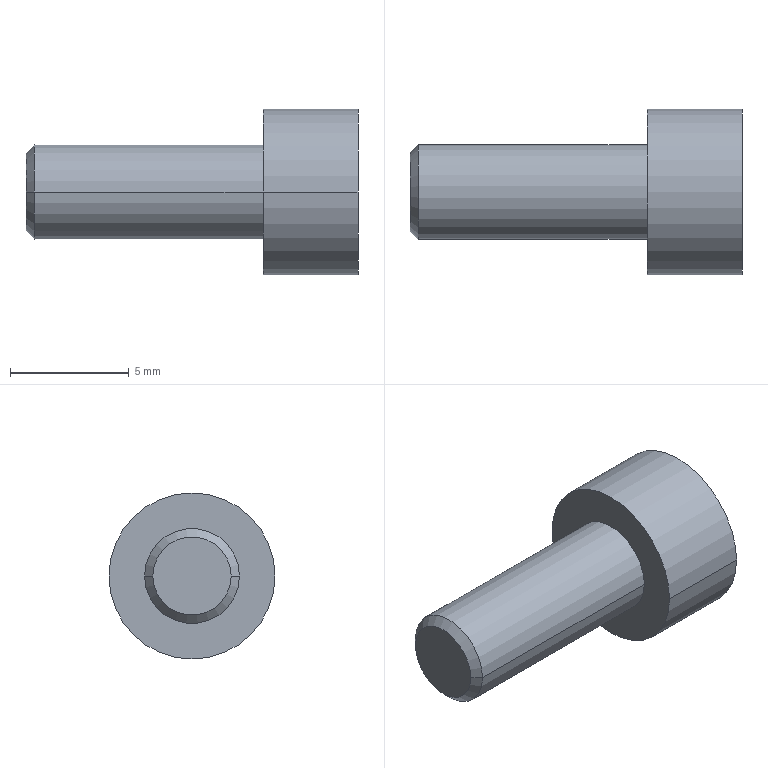Part | STEP file | 4-20.sldasm-Part-224 | 1 solid | 16 faces | box 14 x 7 x 7 mm | volume 258.3 mm3 | plane 10 | cylinder 4 | cone 2 | commonest cylinder face diameters 4 x2 7 x2
STEP:
#1=CARTESIAN_POINT('',(126.065,599.075,-92.493));
#2=VERTEX_POINT('',#1);
#3=CARTESIAN_POINT('',(126.065,595.775,-92.493));
#4=VERTEX_POINT('',#3);
#5=CARTESIAN_POINT('',(126.065,597.425,-92.493));
#6=DIRECTION('',(-1.,0.,0.));
#7=DIRECTION('',(0.,-1.,0.));
#8=AXIS2_PLACEMENT_3D('',#5,#6,#7);
#9=CIRCLE('',#8,1.65);
#10=EDGE_CURVE('',#2,#4,#9,.T.);
#11=ORIENTED_EDGE('',*,*,#10,.F.);
#12=CARTESIAN_POINT('',(126.415,599.425,-92.493));
#13=VERTEX_POINT('',#12);
#14=CARTESIAN_POINT('',(126.415,599.425,-92.493));
#15=DIRECTION('',(0.7071,0.7071,0.));
#16=VECTOR('',#15,1000.);
#17=LINE('',#14,#16);
#18=EDGE_CURVE('',#2,#13,#17,.T.);
#19=ORIENTED_EDGE('',*,*,#18,.T.);
#20=CARTESIAN_POINT('',(126.415,595.425,-92.493));
#21=VERTEX_POINT('',#20);
#22=CARTESIAN_POINT('',(126.415,597.425,-92.493));
#23=DIRECTION('',(1.,0.,0.));
#24=DIRECTION('',(0.,-1.,0.));
#25=AXIS2_PLACEMENT_3D('',#22,#23,#24);
#26=CIRCLE('',#25,2.);
#27=EDGE_CURVE('',#21,#13,#26,.T.);
#28=ORIENTED_EDGE('',*,*,#27,.F.);
#29=CARTESIAN_POINT('',(126.415,595.425,-92.493));
#30=DIRECTION('',(0.7071,-0.7071,0.));
#31=VECTOR('',#30,1000.);
#32=LINE('',#29,#31);
#33=EDGE_CURVE('',#4,#21,#32,.T.);
#34=ORIENTED_EDGE('',*,*,#33,.F.);
#35=EDGE_LOOP('',(#11,#19,#28,#34));
#36=FACE_OUTER_BOUND('',#35,.T.);
#37=CARTESIAN_POINT('',(126.415,597.425,-92.493));
#38=DIRECTION('',(1.,0.,0.));
#39=DIRECTION('',(0.,-1.,0.));
#40=AXIS2_PLACEMENT_3D('',#37,#38,#39);
#41=CONICAL_SURFACE('',#40,2.,0.7854);
#42=ADVANCED_FACE('',(#36),#41,.T.);
#43=CARTESIAN_POINT('',(136.065,593.925,-92.493));
#44=VERTEX_POINT('',#43);
#45=CARTESIAN_POINT('',(136.065,600.925,-92.493));
#46=VERTEX_POINT('',#45);
#47=CARTESIAN_POINT('',(136.065,597.425,-92.493));
#48=DIRECTION('',(1.,0.,0.));
#49=DIRECTION('',(0.,-1.,0.));
#50=AXIS2_PLACEMENT_3D('',#47,#48,#49);
#51=CIRCLE('',#50,3.5);
#52=EDGE_CURVE('',#44,#46,#51,.T.);
#53=ORIENTED_EDGE('',*,*,#52,.T.);
#54=CARTESIAN_POINT('',(140.065,600.925,-92.493));
#55=VERTEX_POINT('',#54);
#56=CARTESIAN_POINT('',(136.065,600.925,-92.493));
#57=DIRECTION('',(1.,0.,0.));
#58=VECTOR('',#57,1000.);
#59=LINE('',#56,#58);
#60=EDGE_CURVE('',#46,#55,#59,.T.);
#61=ORIENTED_EDGE('',*,*,#60,.T.);
#62=CARTESIAN_POINT('',(140.065,593.925,-92.493));
#63=VERTEX_POINT('',#62);
#64=CARTESIAN_POINT('',(140.065,597.425,-92.493));
#65=DIRECTION('',(1.,0.,0.));
#66=DIRECTION('',(0.,-1.,0.));
#67=AXIS2_PLACEMENT_3D('',#64,#65,#66);
#68=CIRCLE('',#67,3.5);
#69=EDGE_CURVE('',#63,#55,#68,.T.);
#70=ORIENTED_EDGE('',*,*,#69,.F.);
#71=CARTESIAN_POINT('',(136.065,593.925,-92.493));
#72=DIRECTION('',(1.,0.,0.));
#73=VECTOR('',#72,1000.);
#74=LINE('',#71,#73);
#75=EDGE_CURVE('',#44,#63,#74,.T.);
#76=ORIENTED_EDGE('',*,*,#75,.F.);
#77=EDGE_LOOP('',(#53,#61,#70,#76));
#78=FACE_OUTER_BOUND('',#77,.T.);
#79=CARTESIAN_POINT('',(136.065,597.425,-92.493));
#80=DIRECTION('',(1.,0.,0.));
#81=DIRECTION('',(0.,-1.,0.));
#82=AXIS2_PLACEMENT_3D('',#79,#80,#81);
#83=CYLINDRICAL_SURFACE('',#82,3.5);
#84=ADVANCED_FACE('',(#78),#83,.T.);
#85=CARTESIAN_POINT('',(136.065,595.425,-92.493));
#86=VERTEX_POINT('',#85);
#87=CARTESIAN_POINT('',(136.065,599.425,-92.493));
#88=VERTEX_POINT('',#87);
#89=CARTESIAN_POINT('',(136.065,597.425,-92.493));
#90=DIRECTION('',(1.,0.,0.));
#91=DIRECTION('',(0.,-1.,0.));
#92=AXIS2_PLACEMENT_3D('',#89,#90,#91);
#93=CIRCLE('',#92,2.);
#94=EDGE_CURVE('',#86,#88,#93,.T.);
#95=ORIENTED_EDGE('',*,*,#94,.F.);
#96=CARTESIAN_POINT('',(136.065,595.425,-92.493));
#97=DIRECTION('',(-1.,0.,0.));
#98=VECTOR('',#97,1000.);
#99=LINE('',#96,#98);
#100=EDGE_CURVE('',#86,#21,#99,.T.);
#101=ORIENTED_EDGE('',*,*,#100,.T.);
#102=ORIENTED_EDGE('',*,*,#27,.T.);
#103=CARTESIAN_POINT('',(136.065,599.425,-92.493));
#104=DIRECTION('',(-1.,0.,0.));
#105=VECTOR('',#104,1000.);
#106=LINE('',#103,#105);
#107=EDGE_CURVE('',#88,#13,#106,.T.);
#108=ORIENTED_EDGE('',*,*,#107,.F.);
#109=EDGE_LOOP('',(#95,#101,#102,#108));
#110=FACE_OUTER_BOUND('',#109,.T.);
#111=CARTESIAN_POINT('',(136.065,597.425,-92.493));
#112=DIRECTION('',(-1.,0.,0.));
#113=DIRECTION('',(0.,1.,0.));
#114=AXIS2_PLACEMENT_3D('',#111,#112,#113);
#115=CYLINDRICAL_SURFACE('',#114,2.);
#116=ADVANCED_FACE('',(#110),#115,.T.);
#117=ORIENTED_EDGE('',*,*,#100,.F.);
#118=CARTESIAN_POINT('',(136.065,597.425,-92.493));
#119=DIRECTION('',(1.,0.,0.));
#120=DIRECTION('',(0.,-1.,0.));
#121=AXIS2_PLACEMENT_3D('',#118,#119,#120);
#122=CIRCLE('',#121,2.);
#123=EDGE_CURVE('',#88,#86,#122,.T.);
#124=ORIENTED_EDGE('',*,*,#123,.F.);
#125=ORIENTED_EDGE('',*,*,#107,.T.);
#126=CARTESIAN_POINT('',(126.415,597.425,-92.493));
#127=DIRECTION('',(1.,0.,0.));
#128=DIRECTION('',(0.,-1.,0.));
#129=AXIS2_PLACEMENT_3D('',#126,#127,#128);
#130=CIRCLE('',#129,2.);
#131=EDGE_CURVE('',#13,#21,#130,.T.);
#132=ORIENTED_EDGE('',*,*,#131,.T.);
#133=EDGE_LOOP('',(#117,#124,#125,#132));
#134=FACE_OUTER_BOUND('',#133,.T.);
#135=CARTESIAN_POINT('',(136.065,597.425,-92.493));
#136=DIRECTION('',(-1.,0.,0.));
#137=DIRECTION('',(0.,1.,0.));
#138=AXIS2_PLACEMENT_3D('',#135,#136,#137);
#139=CYLINDRICAL_SURFACE('',#138,2.);
#140=ADVANCED_FACE('',(#134),#139,.T.);
#141=CARTESIAN_POINT('',(126.065,597.425,-92.493));
#142=DIRECTION('',(-1.,0.,0.));
#143=DIRECTION('',(0.,-1.,0.));
#144=AXIS2_PLACEMENT_3D('',#141,#142,#143);
#145=CIRCLE('',#144,1.65);
#146=EDGE_CURVE('',#4,#2,#145,.T.);
#147=ORIENTED_EDGE('',*,*,#146,.T.);
#148=ORIENTED_EDGE('',*,*,#10,.T.);
#149=EDGE_LOOP('',(#147,#148));
#150=FACE_OUTER_BOUND('',#149,.T.);
#151=CARTESIAN_POINT('',(126.065,597.425,-92.493));
#152=DIRECTION('',(1.,0.,0.));
#153=DIRECTION('',(0.,-1.,0.));
#154=AXIS2_PLACEMENT_3D('',#151,#152,#153);
#155=PLANE('',#154);
#156=ADVANCED_FACE('',(#150),#155,.F.);
#157=ORIENTED_EDGE('',*,*,#52,.F.);
#158=CARTESIAN_POINT('',(136.065,597.425,-92.493));
#159=DIRECTION('',(1.,0.,0.));
#160=DIRECTION('',(0.,-1.,0.));
#161=AXIS2_PLACEMENT_3D('',#158,#159,#160);
#162=CIRCLE('',#161,3.5);
#163=EDGE_CURVE('',#46,#44,#162,.T.);
#164=ORIENTED_EDGE('',*,*,#163,.F.);
#165=EDGE_LOOP('',(#157,#164));
#166=FACE_OUTER_BOUND('',#165,.T.);
#167=ORIENTED_EDGE('',*,*,#123,.T.);
#168=ORIENTED_EDGE('',*,*,#94,.T.);
#169=EDGE_LOOP('',(#167,#168));
#170=FACE_BOUND('',#169,.T.);
#171=CARTESIAN_POINT('',(136.065,597.425,-92.493));
#172=DIRECTION('',(-1.,0.,0.));
#173=DIRECTION('',(0.,1.,0.));
#174=AXIS2_PLACEMENT_3D('',#171,#172,#173);
#175=PLANE('',#174);
#176=ADVANCED_FACE('',(#166,#170),#175,.T.);
#177=CARTESIAN_POINT('',(140.065,598.291,-90.993));
#178=VERTEX_POINT('',#177);
#179=CARTESIAN_POINT('',(140.065,596.559,-90.993));
#180=VERTEX_POINT('',#179);
#181=CARTESIAN_POINT('',(140.065,598.291,-90.993));
#182=DIRECTION('',(0.,-1.,0.));
#183=VECTOR('',#182,1000.);
#184=LINE('',#181,#183);
#185=EDGE_CURVE('',#178,#180,#184,.T.);
#186=ORIENTED_EDGE('',*,*,#185,.F.);
#187=CARTESIAN_POINT('',(140.065,599.157,-92.493));
#188=VERTEX_POINT('',#187);
#189=CARTESIAN_POINT('',(140.065,599.157,-92.493));
#190=DIRECTION('',(0.,-0.5,0.866));
#191=VECTOR('',#190,1000.);
#192=LINE('',#189,#191);
#193=EDGE_CURVE('',#188,#178,#192,.T.);
#194=ORIENTED_EDGE('',*,*,#193,.F.);
#195=CARTESIAN_POINT('',(140.065,598.291,-93.993));
#196=VERTEX_POINT('',#195);
#197=CARTESIAN_POINT('',(140.065,598.291,-93.993));
#198=DIRECTION('',(0.,0.5,0.866));
#199=VECTOR('',#198,1000.);
#200=LINE('',#197,#199);
#201=EDGE_CURVE('',#196,#188,#200,.T.);
#202=ORIENTED_EDGE('',*,*,#201,.F.);
#203=CARTESIAN_POINT('',(140.065,596.559,-93.993));
#204=VERTEX_POINT('',#203);
#205=CARTESIAN_POINT('',(140.065,596.559,-93.993));
#206=DIRECTION('',(0.,1.,0.));
#207=VECTOR('',#206,1000.);
#208=LINE('',#205,#207);
#209=EDGE_CURVE('',#204,#196,#208,.T.);
#210=ORIENTED_EDGE('',*,*,#209,.F.);
#211=CARTESIAN_POINT('',(140.065,595.693,-92.493));
#212=VERTEX_POINT('',#211);
#213=CARTESIAN_POINT('',(140.065,595.693,-92.493));
#214=DIRECTION('',(0.,0.5,-0.866));
#215=VECTOR('',#214,1000.);
#216=LINE('',#213,#215);
#217=EDGE_CURVE('',#212,#204,#216,.T.);
#218=ORIENTED_EDGE('',*,*,#217,.F.);
#219=CARTESIAN_POINT('',(140.065,596.559,-90.993));
#220=DIRECTION('',(0.,-0.5,-0.866));
#221=VECTOR('',#220,1000.);
#222=LINE('',#219,#221);
#223=EDGE_CURVE('',#180,#212,#222,.T.);
#224=ORIENTED_EDGE('',*,*,#223,.F.);
#225=EDGE_LOOP('',(#186,#194,#202,#210,#218,#224));
#226=FACE_BOUND('',#225,.T.);
#227=ORIENTED_EDGE('',*,*,#69,.T.);
#228=CARTESIAN_POINT('',(140.065,597.425,-92.493));
#229=DIRECTION('',(1.,0.,0.));
#230=DIRECTION('',(0.,-1.,0.));
#231=AXIS2_PLACEMENT_3D('',#228,#229,#230);
#232=CIRCLE('',#231,3.5);
#233=EDGE_CURVE('',#55,#63,#232,.T.);
#234=ORIENTED_EDGE('',*,*,#233,.T.);
#235=EDGE_LOOP('',(#227,#234));
#236=FACE_OUTER_BOUND('',#235,.T.);
#237=CARTESIAN_POINT('',(140.065,597.425,-92.493));
#238=DIRECTION('',(1.,0.,0.));
#239=DIRECTION('',(0.,-1.,0.));
#240=AXIS2_PLACEMENT_3D('',#237,#238,#239);
#241=PLANE('',#240);
#242=ADVANCED_FACE('',(#226,#236),#241,.T.);
#243=ORIENTED_EDGE('',*,*,#60,.F.);
#244=ORIENTED_EDGE('',*,*,#163,.T.);
#245=ORIENTED_EDGE('',*,*,#75,.T.);
#246=ORIENTED_EDGE('',*,*,#233,.F.);
#247=EDGE_LOOP('',(#243,#244,#245,#246));
#248=FACE_OUTER_BOUND('',#247,.T.);
#249=CARTESIAN_POINT('',(136.065,597.425,-92.493));
#250=DIRECTION('',(1.,0.,0.));
#251=DIRECTION('',(0.,-1.,0.));
#252=AXIS2_PLACEMENT_3D('',#249,#250,#251);
#253=CYLINDRICAL_SURFACE('',#252,3.5);
#254=ADVANCED_FACE('',(#248),#253,.T.);
#255=ORIENTED_EDGE('',*,*,#18,.F.);
#256=ORIENTED_EDGE('',*,*,#146,.F.);
#257=ORIENTED_EDGE('',*,*,#33,.T.);
#258=ORIENTED_EDGE('',*,*,#131,.F.);
#259=EDGE_LOOP('',(#255,#256,#257,#258));
#260=FACE_OUTER_BOUND('',#259,.T.);
#261=CARTESIAN_POINT('',(126.415,597.425,-92.493));
#262=DIRECTION('',(1.,0.,0.));
#263=DIRECTION('',(0.,-1.,0.));
#264=AXIS2_PLACEMENT_3D('',#261,#262,#263);
#265=CONICAL_SURFACE('',#264,2.,0.7854);
#266=ADVANCED_FACE('',(#260),#265,.T.);
#267=ORIENTED_EDGE('',*,*,#185,.T.);
#268=CARTESIAN_POINT('',(137.425,596.559,-90.993));
#269=VERTEX_POINT('',#268);
#270=CARTESIAN_POINT('',(137.425,596.559,-90.993));
#271=DIRECTION('',(1.,0.,0.));
#272=VECTOR('',#271,1000.);
#273=LINE('',#270,#272);
#274=EDGE_CURVE('',#269,#180,#273,.T.);
#275=ORIENTED_EDGE('',*,*,#274,.F.);
#276=CARTESIAN_POINT('',(137.425,598.291,-90.993));
#277=VERTEX_POINT('',#276);
#278=CARTESIAN_POINT('',(137.425,598.291,-90.993));
#279=DIRECTION('',(0.,-1.,0.));
#280=VECTOR('',#279,1000.);
#281=LINE('',#278,#280);
#282=EDGE_CURVE('',#277,#269,#281,.T.);
#283=ORIENTED_EDGE('',*,*,#282,.F.);
#284=CARTESIAN_POINT('',(137.425,598.291,-90.993));
#285=DIRECTION('',(1.,0.,0.));
#286=VECTOR('',#285,1000.);
#287=LINE('',#284,#286);
#288=EDGE_CURVE('',#277,#178,#287,.T.);
#289=ORIENTED_EDGE('',*,*,#288,.T.);
#290=EDGE_LOOP('',(#267,#275,#283,#289));
#291=FACE_OUTER_BOUND('',#290,.T.);
#292=CARTESIAN_POINT('',(137.425,598.291,-90.993));
#293=DIRECTION('',(0.,0.,1.));
#294=DIRECTION('',(-1.,0.,0.));
#295=AXIS2_PLACEMENT_3D('',#292,#293,#294);
#296=PLANE('',#295);
#297=ADVANCED_FACE('',(#291),#296,.F.);
#298=ORIENTED_EDGE('',*,*,#223,.T.);
#299=CARTESIAN_POINT('',(137.425,595.693,-92.493));
#300=VERTEX_POINT('',#299);
#301=CARTESIAN_POINT('',(137.425,595.693,-92.493));
#302=DIRECTION('',(1.,0.,0.));
#303=VECTOR('',#302,1000.);
#304=LINE('',#301,#303);
#305=EDGE_CURVE('',#300,#212,#304,.T.);
#306=ORIENTED_EDGE('',*,*,#305,.F.);
#307=CARTESIAN_POINT('',(137.425,596.559,-90.993));
#308=DIRECTION('',(0.,-0.5,-0.866));
#309=VECTOR('',#308,1000.);
#310=LINE('',#307,#309);
#311=EDGE_CURVE('',#269,#300,#310,.T.);
#312=ORIENTED_EDGE('',*,*,#311,.F.);
#313=ORIENTED_EDGE('',*,*,#274,.T.);
#314=EDGE_LOOP('',(#298,#306,#312,#313));
#315=FACE_OUTER_BOUND('',#314,.T.);
#316=CARTESIAN_POINT('',(137.425,596.559,-90.993));
#317=DIRECTION('',(0.,-0.866,0.5));
#318=DIRECTION('',(0.,-0.5,-0.866));
#319=AXIS2_PLACEMENT_3D('',#316,#317,#318);
#320=PLANE('',#319);
#321=ADVANCED_FACE('',(#315),#320,.F.);
#322=ORIENTED_EDGE('',*,*,#217,.T.);
#323=CARTESIAN_POINT('',(137.425,596.559,-93.993));
#324=VERTEX_POINT('',#323);
#325=CARTESIAN_POINT('',(137.425,596.559,-93.993));
#326=DIRECTION('',(1.,0.,0.));
#327=VECTOR('',#326,1000.);
#328=LINE('',#325,#327);
#329=EDGE_CURVE('',#324,#204,#328,.T.);
#330=ORIENTED_EDGE('',*,*,#329,.F.);
#331=CARTESIAN_POINT('',(137.425,595.693,-92.493));
#332=DIRECTION('',(0.,0.5,-0.866));
#333=VECTOR('',#332,1000.);
#334=LINE('',#331,#333);
#335=EDGE_CURVE('',#300,#324,#334,.T.);
#336=ORIENTED_EDGE('',*,*,#335,.F.);
#337=ORIENTED_EDGE('',*,*,#305,.T.);
#338=EDGE_LOOP('',(#322,#330,#336,#337));
#339=FACE_OUTER_BOUND('',#338,.T.);
#340=CARTESIAN_POINT('',(137.425,595.693,-92.493));
#341=DIRECTION('',(0.,-0.866,-0.5));
#342=DIRECTION('',(0.,0.5,-0.866));
#343=AXIS2_PLACEMENT_3D('',#340,#341,#342);
#344=PLANE('',#343);
#345=ADVANCED_FACE('',(#339),#344,.F.);
#346=ORIENTED_EDGE('',*,*,#209,.T.);
#347=CARTESIAN_POINT('',(137.425,598.291,-93.993));
#348=VERTEX_POINT('',#347);
#349=CARTESIAN_POINT('',(137.425,598.291,-93.993));
#350=DIRECTION('',(1.,0.,0.));
#351=VECTOR('',#350,1000.);
#352=LINE('',#349,#351);
#353=EDGE_CURVE('',#348,#196,#352,.T.);
#354=ORIENTED_EDGE('',*,*,#353,.F.);
#355=CARTESIAN_POINT('',(137.425,596.559,-93.993));
#356=DIRECTION('',(0.,1.,0.));
#357=VECTOR('',#356,1000.);
#358=LINE('',#355,#357);
#359=EDGE_CURVE('',#324,#348,#358,.T.);
#360=ORIENTED_EDGE('',*,*,#359,.F.);
#361=ORIENTED_EDGE('',*,*,#329,.T.);
#362=EDGE_LOOP('',(#346,#354,#360,#361));
#363=FACE_OUTER_BOUND('',#362,.T.);
#364=CARTESIAN_POINT('',(137.425,596.559,-93.993));
#365=DIRECTION('',(0.,0.,-1.));
#366=DIRECTION('',(1.,0.,0.));
#367=AXIS2_PLACEMENT_3D('',#364,#365,#366);
#368=PLANE('',#367);
#369=ADVANCED_FACE('',(#363),#368,.F.);
#370=ORIENTED_EDGE('',*,*,#201,.T.);
#371=CARTESIAN_POINT('',(137.425,599.157,-92.493));
#372=VERTEX_POINT('',#371);
#373=CARTESIAN_POINT('',(137.425,599.157,-92.493));
#374=DIRECTION('',(1.,0.,0.));
#375=VECTOR('',#374,1000.);
#376=LINE('',#373,#375);
#377=EDGE_CURVE('',#372,#188,#376,.T.);
#378=ORIENTED_EDGE('',*,*,#377,.F.);
#379=CARTESIAN_POINT('',(137.425,598.291,-93.993));
#380=DIRECTION('',(0.,0.5,0.866));
#381=VECTOR('',#380,1000.);
#382=LINE('',#379,#381);
#383=EDGE_CURVE('',#348,#372,#382,.T.);
#384=ORIENTED_EDGE('',*,*,#383,.F.);
#385=ORIENTED_EDGE('',*,*,#353,.T.);
#386=EDGE_LOOP('',(#370,#378,#384,#385));
#387=FACE_OUTER_BOUND('',#386,.T.);
#388=CARTESIAN_POINT('',(137.425,598.291,-93.993));
#389=DIRECTION('',(0.,0.866,-0.5));
#390=DIRECTION('',(0.,0.5,0.866));
#391=AXIS2_PLACEMENT_3D('',#388,#389,#390);
#392=PLANE('',#391);
#393=ADVANCED_FACE('',(#387),#392,.F.);
#394=ORIENTED_EDGE('',*,*,#193,.T.);
#395=ORIENTED_EDGE('',*,*,#288,.F.);
#396=CARTESIAN_POINT('',(137.425,599.157,-92.493));
#397=DIRECTION('',(0.,-0.5,0.866));
#398=VECTOR('',#397,1000.);
#399=LINE('',#396,#398);
#400=EDGE_CURVE('',#372,#277,#399,.T.);
#401=ORIENTED_EDGE('',*,*,#400,.F.);
#402=ORIENTED_EDGE('',*,*,#377,.T.);
#403=EDGE_LOOP('',(#394,#395,#401,#402));
#404=FACE_OUTER_BOUND('',#403,.T.);
#405=CARTESIAN_POINT('',(137.425,599.157,-92.493));
#406=DIRECTION('',(0.,0.866,0.5));
#407=DIRECTION('',(0.,-0.5,0.866));
#408=AXIS2_PLACEMENT_3D('',#405,#406,#407);
#409=PLANE('',#408);
#410=ADVANCED_FACE('',(#404),#409,.F.);
#411=ORIENTED_EDGE('',*,*,#282,.T.);
#412=ORIENTED_EDGE('',*,*,#311,.T.);
#413=ORIENTED_EDGE('',*,*,#335,.T.);
#414=ORIENTED_EDGE('',*,*,#359,.T.);
#415=ORIENTED_EDGE('',*,*,#383,.T.);
#416=ORIENTED_EDGE('',*,*,#400,.T.);
#417=EDGE_LOOP('',(#411,#412,#413,#414,#415,#416));
#418=FACE_OUTER_BOUND('',#417,.T.);
#419=CARTESIAN_POINT('',(137.425,596.559,-90.993));
#420=DIRECTION('',(1.,0.,0.));
#421=DIRECTION('',(0.,-1.,0.));
#422=AXIS2_PLACEMENT_3D('',#419,#420,#421);
#423=PLANE('',#422);
#424=ADVANCED_FACE('',(#418),#423,.T.);
#425=CLOSED_SHELL('',(#42,#84,#116,#140,#156,#176,#242,#254,#266,#297,#321,#345,#369,#393,#410,#424));
#426=MANIFOLD_SOLID_BREP('',#425);
#427=CARTESIAN_POINT('',(0.,0.,0.));
#428=DIRECTION('',(0.,0.,1.));
#429=DIRECTION('',(1.,0.,0.));
#430=AXIS2_PLACEMENT_3D('',#427,#428,#429);
#431=(LENGTH_UNIT()NAMED_UNIT(*)SI_UNIT(.MILLI.,.METRE.));
#432=UNCERTAINTY_MEASURE_WITH_UNIT(LENGTH_MEASURE(0.00001),#431,'','');
#433=(NAMED_UNIT(*)PLANE_ANGLE_UNIT()SI_UNIT($,.RADIAN.));
#434=(NAMED_UNIT(*)SI_UNIT($,.STERADIAN.)SOLID_ANGLE_UNIT());
#435=(GEOMETRIC_REPRESENTATION_CONTEXT(3)GLOBAL_UNCERTAINTY_ASSIGNED_CONTEXT((#432))GLOBAL_UNIT_ASSIGNED_CONTEXT((#431,#433,#434))REPRESENTATION_CONTEXT('',''));
#436=ADVANCED_BREP_SHAPE_REPRESENTATION('',(#426,#430),#435);